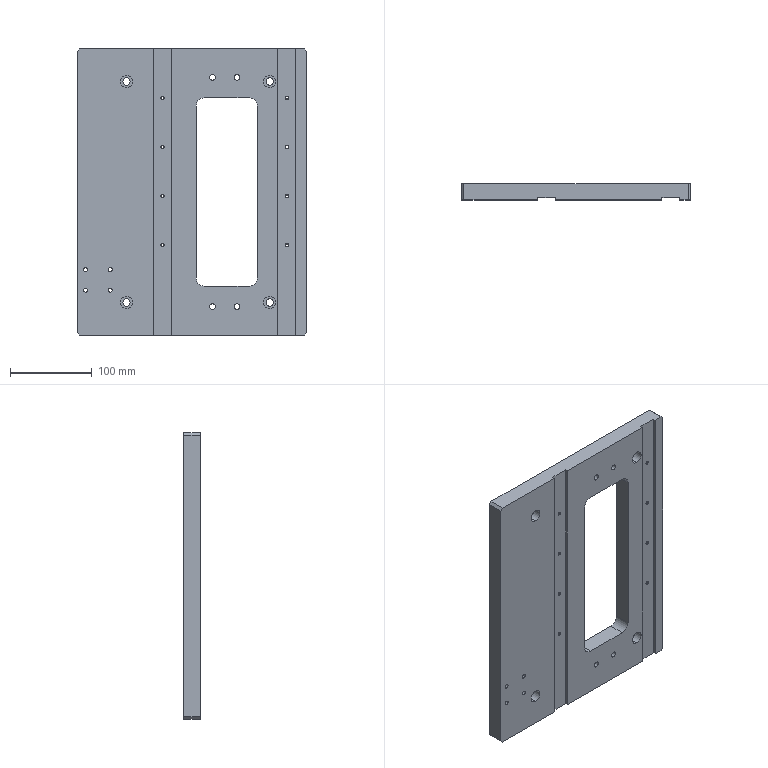Part | SolidWorks | features HoleWzd 6, Chamfer 1, Extrusion 1, Fillet 1, ICE 1 | 1 solid | 106 faces | box 280 x 20 x 350 mm | volume 1546665 mm3 | cylinder 60 | plane 30 | cone 16 | commonest cylinder face diameters 3.3 x16 5 x8 6.8 x8 9 x8 15 x8 20 x4